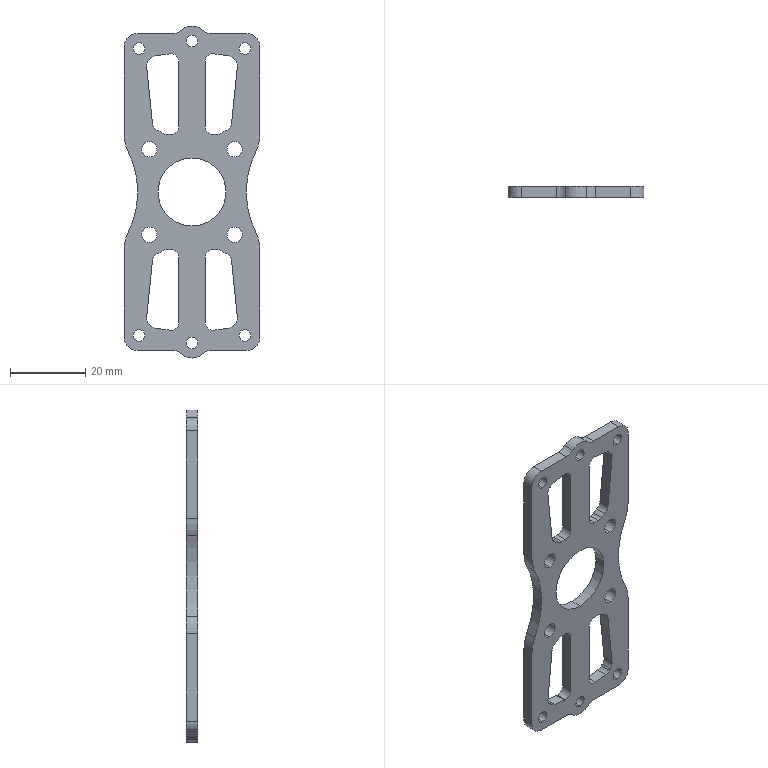Part | SolidWorks | features Fillet 3, Extrusion 1, ICE 1 | 1 solid | 99 faces | box 36 x 3 x 88 mm | volume 5789 mm3 | cylinder 73 | plane 26 | commonest cylinder face diameters 4 x26 3.1 x12 4.05 x8 7 x8 8 x7 11 x4